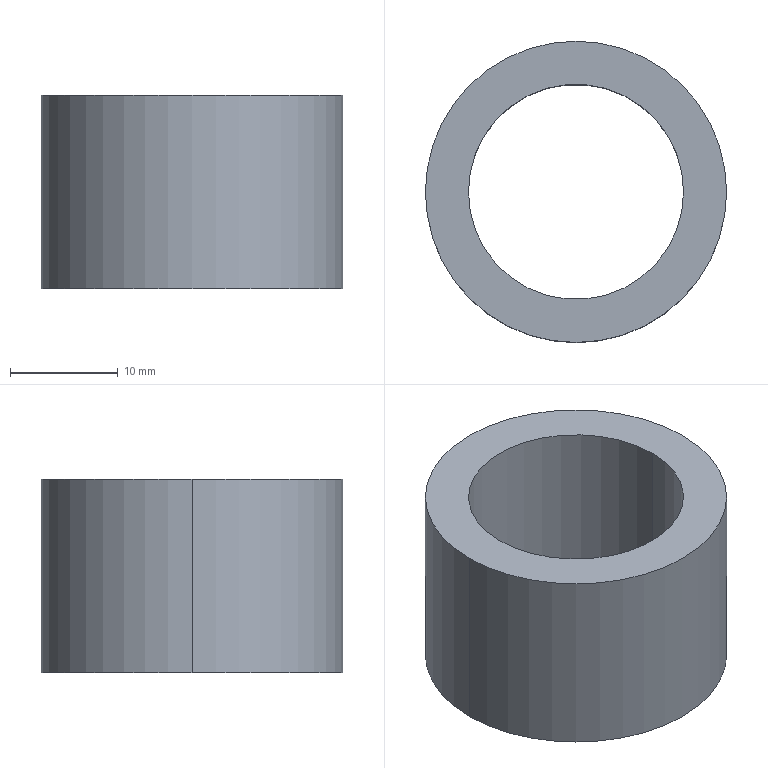Part | STEP file | Large pulley shaft collar | 1 solid | 6 faces | box 28 x 28 x 18 mm | volume 5429 mm3 | cylinder 4 | plane 2 | commonest cylinder face diameters 20 x2 28 x2
STEP:
#1=CARTESIAN_POINT('',(-10.,0.,18.));
#2=VERTEX_POINT('',#1);
#3=CARTESIAN_POINT('',(10.,0.,18.));
#4=VERTEX_POINT('',#3);
#5=CARTESIAN_POINT('',(0.,0.,18.));
#6=DIRECTION('',(0.,0.,1.));
#7=DIRECTION('',(1.,0.,0.));
#8=AXIS2_PLACEMENT_3D('',#5,#6,#7);
#9=CIRCLE('',#8,10.);
#10=EDGE_CURVE('',#2,#4,#9,.T.);
#11=ORIENTED_EDGE('',*,*,#10,.T.);
#12=CARTESIAN_POINT('',(10.,0.,0.));
#13=VERTEX_POINT('',#12);
#14=CARTESIAN_POINT('',(10.,0.,18.));
#15=DIRECTION('',(0.,0.,-1.));
#16=VECTOR('',#15,1000.);
#17=LINE('',#14,#16);
#18=EDGE_CURVE('',#4,#13,#17,.T.);
#19=ORIENTED_EDGE('',*,*,#18,.T.);
#20=CARTESIAN_POINT('',(-10.,0.,0.));
#21=VERTEX_POINT('',#20);
#22=CARTESIAN_POINT('',(0.,0.,0.));
#23=DIRECTION('',(0.,0.,1.));
#24=DIRECTION('',(1.,0.,0.));
#25=AXIS2_PLACEMENT_3D('',#22,#23,#24);
#26=CIRCLE('',#25,10.);
#27=EDGE_CURVE('',#21,#13,#26,.T.);
#28=ORIENTED_EDGE('',*,*,#27,.F.);
#29=CARTESIAN_POINT('',(-10.,0.,18.));
#30=DIRECTION('',(0.,0.,-1.));
#31=VECTOR('',#30,1000.);
#32=LINE('',#29,#31);
#33=EDGE_CURVE('',#2,#21,#32,.T.);
#34=ORIENTED_EDGE('',*,*,#33,.F.);
#35=EDGE_LOOP('',(#11,#19,#28,#34));
#36=FACE_OUTER_BOUND('',#35,.T.);
#37=CARTESIAN_POINT('',(0.,0.,18.));
#38=DIRECTION('',(0.,0.,-1.));
#39=DIRECTION('',(-1.,0.,0.));
#40=AXIS2_PLACEMENT_3D('',#37,#38,#39);
#41=CYLINDRICAL_SURFACE('',#40,10.);
#42=ADVANCED_FACE('',(#36),#41,.F.);
#43=CARTESIAN_POINT('',(14.,0.,18.));
#44=VERTEX_POINT('',#43);
#45=CARTESIAN_POINT('',(-14.,0.,18.));
#46=VERTEX_POINT('',#45);
#47=CARTESIAN_POINT('',(0.,0.,18.));
#48=DIRECTION('',(0.,0.,1.));
#49=DIRECTION('',(1.,0.,0.));
#50=AXIS2_PLACEMENT_3D('',#47,#48,#49);
#51=CIRCLE('',#50,14.);
#52=EDGE_CURVE('',#44,#46,#51,.T.);
#53=ORIENTED_EDGE('',*,*,#52,.F.);
#54=CARTESIAN_POINT('',(14.,0.,0.));
#55=VERTEX_POINT('',#54);
#56=CARTESIAN_POINT('',(14.,0.,18.));
#57=DIRECTION('',(0.,0.,-1.));
#58=VECTOR('',#57,1000.);
#59=LINE('',#56,#58);
#60=EDGE_CURVE('',#44,#55,#59,.T.);
#61=ORIENTED_EDGE('',*,*,#60,.T.);
#62=CARTESIAN_POINT('',(-14.,0.,0.));
#63=VERTEX_POINT('',#62);
#64=CARTESIAN_POINT('',(0.,0.,0.));
#65=DIRECTION('',(0.,0.,1.));
#66=DIRECTION('',(1.,0.,0.));
#67=AXIS2_PLACEMENT_3D('',#64,#65,#66);
#68=CIRCLE('',#67,14.);
#69=EDGE_CURVE('',#55,#63,#68,.T.);
#70=ORIENTED_EDGE('',*,*,#69,.T.);
#71=CARTESIAN_POINT('',(-14.,0.,18.));
#72=DIRECTION('',(0.,0.,-1.));
#73=VECTOR('',#72,1000.);
#74=LINE('',#71,#73);
#75=EDGE_CURVE('',#46,#63,#74,.T.);
#76=ORIENTED_EDGE('',*,*,#75,.F.);
#77=EDGE_LOOP('',(#53,#61,#70,#76));
#78=FACE_OUTER_BOUND('',#77,.T.);
#79=CARTESIAN_POINT('',(0.,0.,18.));
#80=DIRECTION('',(0.,0.,-1.));
#81=DIRECTION('',(-1.,0.,0.));
#82=AXIS2_PLACEMENT_3D('',#79,#80,#81);
#83=CYLINDRICAL_SURFACE('',#82,14.);
#84=ADVANCED_FACE('',(#78),#83,.T.);
#85=CARTESIAN_POINT('',(0.,0.,18.));
#86=DIRECTION('',(0.,0.,1.));
#87=DIRECTION('',(1.,0.,0.));
#88=AXIS2_PLACEMENT_3D('',#85,#86,#87);
#89=CIRCLE('',#88,14.);
#90=EDGE_CURVE('',#46,#44,#89,.T.);
#91=ORIENTED_EDGE('',*,*,#90,.T.);
#92=ORIENTED_EDGE('',*,*,#52,.T.);
#93=EDGE_LOOP('',(#91,#92));
#94=FACE_OUTER_BOUND('',#93,.T.);
#95=ORIENTED_EDGE('',*,*,#10,.F.);
#96=CARTESIAN_POINT('',(0.,0.,18.));
#97=DIRECTION('',(0.,0.,1.));
#98=DIRECTION('',(1.,0.,0.));
#99=AXIS2_PLACEMENT_3D('',#96,#97,#98);
#100=CIRCLE('',#99,10.);
#101=EDGE_CURVE('',#4,#2,#100,.T.);
#102=ORIENTED_EDGE('',*,*,#101,.F.);
#103=EDGE_LOOP('',(#95,#102));
#104=FACE_BOUND('',#103,.T.);
#105=CARTESIAN_POINT('',(0.,0.,18.));
#106=DIRECTION('',(0.,0.,1.));
#107=DIRECTION('',(1.,0.,0.));
#108=AXIS2_PLACEMENT_3D('',#105,#106,#107);
#109=PLANE('',#108);
#110=ADVANCED_FACE('',(#94,#104),#109,.T.);
#111=CARTESIAN_POINT('',(0.,0.,0.));
#112=DIRECTION('',(0.,0.,1.));
#113=DIRECTION('',(1.,0.,0.));
#114=AXIS2_PLACEMENT_3D('',#111,#112,#113);
#115=CIRCLE('',#114,14.);
#116=EDGE_CURVE('',#63,#55,#115,.T.);
#117=ORIENTED_EDGE('',*,*,#116,.F.);
#118=ORIENTED_EDGE('',*,*,#69,.F.);
#119=EDGE_LOOP('',(#117,#118));
#120=FACE_OUTER_BOUND('',#119,.T.);
#121=ORIENTED_EDGE('',*,*,#27,.T.);
#122=CARTESIAN_POINT('',(0.,0.,0.));
#123=DIRECTION('',(0.,0.,1.));
#124=DIRECTION('',(1.,0.,0.));
#125=AXIS2_PLACEMENT_3D('',#122,#123,#124);
#126=CIRCLE('',#125,10.);
#127=EDGE_CURVE('',#13,#21,#126,.T.);
#128=ORIENTED_EDGE('',*,*,#127,.T.);
#129=EDGE_LOOP('',(#121,#128));
#130=FACE_BOUND('',#129,.T.);
#131=CARTESIAN_POINT('',(0.,0.,0.));
#132=DIRECTION('',(0.,0.,1.));
#133=DIRECTION('',(1.,0.,0.));
#134=AXIS2_PLACEMENT_3D('',#131,#132,#133);
#135=PLANE('',#134);
#136=ADVANCED_FACE('',(#120,#130),#135,.F.);
#137=ORIENTED_EDGE('',*,*,#60,.F.);
#138=ORIENTED_EDGE('',*,*,#90,.F.);
#139=ORIENTED_EDGE('',*,*,#75,.T.);
#140=ORIENTED_EDGE('',*,*,#116,.T.);
#141=EDGE_LOOP('',(#137,#138,#139,#140));
#142=FACE_OUTER_BOUND('',#141,.T.);
#143=CARTESIAN_POINT('',(0.,0.,18.));
#144=DIRECTION('',(0.,0.,-1.));
#145=DIRECTION('',(-1.,0.,0.));
#146=AXIS2_PLACEMENT_3D('',#143,#144,#145);
#147=CYLINDRICAL_SURFACE('',#146,14.);
#148=ADVANCED_FACE('',(#142),#147,.T.);
#149=ORIENTED_EDGE('',*,*,#18,.F.);
#150=ORIENTED_EDGE('',*,*,#101,.T.);
#151=ORIENTED_EDGE('',*,*,#33,.T.);
#152=ORIENTED_EDGE('',*,*,#127,.F.);
#153=EDGE_LOOP('',(#149,#150,#151,#152));
#154=FACE_OUTER_BOUND('',#153,.T.);
#155=CARTESIAN_POINT('',(0.,0.,18.));
#156=DIRECTION('',(0.,0.,-1.));
#157=DIRECTION('',(-1.,0.,0.));
#158=AXIS2_PLACEMENT_3D('',#155,#156,#157);
#159=CYLINDRICAL_SURFACE('',#158,10.);
#160=ADVANCED_FACE('',(#154),#159,.F.);
#161=CLOSED_SHELL('',(#42,#84,#110,#136,#148,#160));
#162=MANIFOLD_SOLID_BREP('',#161);
#163=CARTESIAN_POINT('',(0.,0.,0.));
#164=DIRECTION('',(0.,0.,1.));
#165=DIRECTION('',(1.,0.,0.));
#166=AXIS2_PLACEMENT_3D('',#163,#164,#165);
#167=(LENGTH_UNIT()NAMED_UNIT(*)SI_UNIT(.MILLI.,.METRE.));
#168=UNCERTAINTY_MEASURE_WITH_UNIT(LENGTH_MEASURE(0.00001),#167,'','');
#169=(NAMED_UNIT(*)PLANE_ANGLE_UNIT()SI_UNIT($,.RADIAN.));
#170=(NAMED_UNIT(*)SI_UNIT($,.STERADIAN.)SOLID_ANGLE_UNIT());
#171=(GEOMETRIC_REPRESENTATION_CONTEXT(3)GLOBAL_UNCERTAINTY_ASSIGNED_CONTEXT((#168))GLOBAL_UNIT_ASSIGNED_CONTEXT((#167,#169,#170))REPRESENTATION_CONTEXT('',''));
#172=ADVANCED_BREP_SHAPE_REPRESENTATION('',(#162,#166),#171);